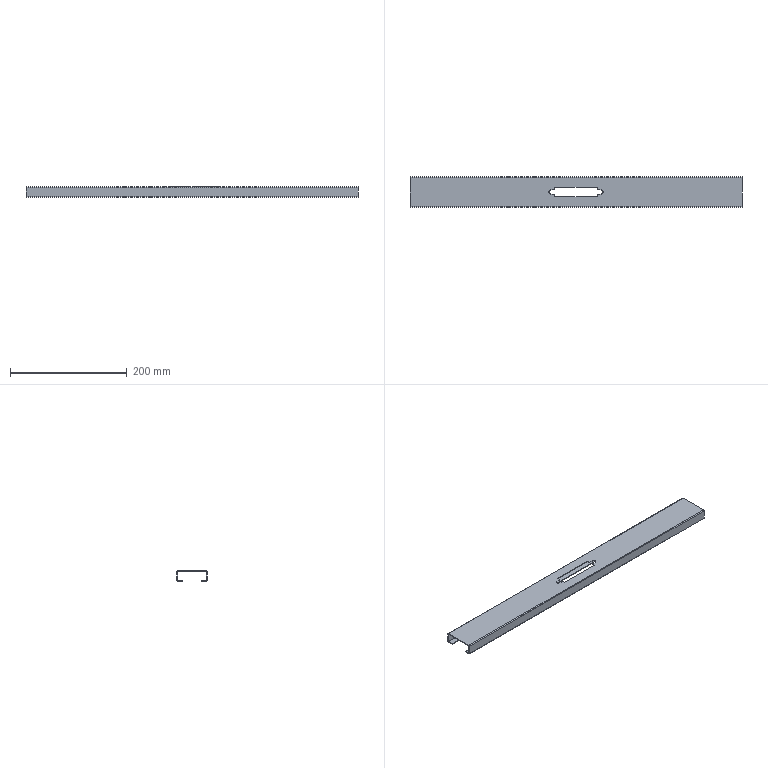Part | STEP file | FHD-021-007-A TZD10S drawer 1 | 1 solid | 34 faces | box 569.6 x 52 x 18 mm | volume 67956 mm3 | plane 24 | cylinder 10 | commonest cylinder face diameters 0.4 x4 2.8 x4 7 x2